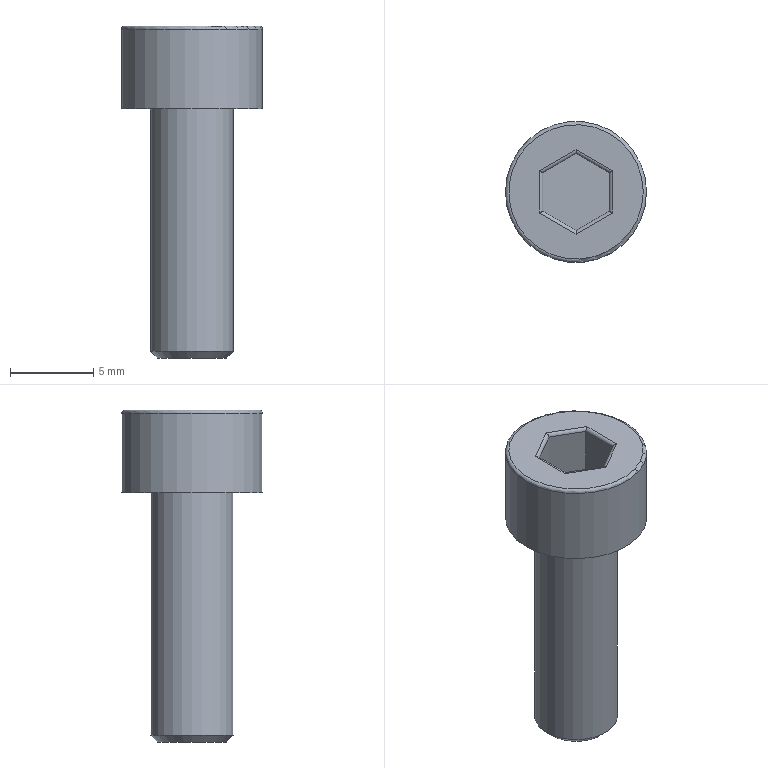Part | STEP file | 200 mesh_id130_x | 1 solid | 20 faces | box 8.5 x 8.5 x 20 mm | volume 535.142 mm3 | plane 10 | cylinder 8 | torus 1 | cone 1 | commonest cylinder face diameters 0.4 x6 5 x1 8.5 x1
STEP:
#1=CARTESIAN_POINT('',(-17018.123,-3964.269,66.658));
#2=VERTEX_POINT('',#1);
#3=CARTESIAN_POINT('',(-17015.623,-3964.269,66.658));
#4=DIRECTION('',(0.,0.,1.));
#5=DIRECTION('',(-1.,0.,0.));
#6=AXIS2_PLACEMENT_3D('',#3,#4,#5);
#7=CIRCLE('',#6,2.5);
#8=EDGE_CURVE('',#2,#2,#7,.T.);
#9=ORIENTED_EDGE('',*,*,#8,.T.);
#10=EDGE_LOOP('',(#9));
#11=FACE_BOUND('',#10,.T.);
#12=CARTESIAN_POINT('',(-17018.123,-3964.269,81.258));
#13=VERTEX_POINT('',#12);
#14=CARTESIAN_POINT('',(-17015.623,-3964.269,81.258));
#15=DIRECTION('',(0.,0.,1.));
#16=DIRECTION('',(-1.,0.,0.));
#17=AXIS2_PLACEMENT_3D('',#14,#15,#16);
#18=CIRCLE('',#17,2.5);
#19=EDGE_CURVE('',#13,#13,#18,.T.);
#20=ORIENTED_EDGE('',*,*,#19,.F.);
#21=EDGE_LOOP('',(#20));
#22=FACE_BOUND('',#21,.T.);
#23=CARTESIAN_POINT('',(-17015.623,-3964.269,81.258));
#24=DIRECTION('',(0.,0.,-1.));
#25=DIRECTION('',(1.,0.,0.));
#26=AXIS2_PLACEMENT_3D('',#23,#24,#25);
#27=CYLINDRICAL_SURFACE('',#26,2.5);
#28=ADVANCED_FACE('',(#11,#22),#27,.T.);
#29=CARTESIAN_POINT('',(-17015.623,-3961.729,86.258));
#30=VERTEX_POINT('',#29);
#31=CARTESIAN_POINT('',(-17013.423,-3962.999,86.258));
#32=VERTEX_POINT('',#31);
#33=CARTESIAN_POINT('',(-17013.523,-3962.941,86.258));
#34=DIRECTION('',(0.866,-0.5,0.));
#35=VECTOR('',#34,1.);
#36=LINE('',#33,#35);
#37=EDGE_CURVE('',#30,#32,#36,.T.);
#38=ORIENTED_EDGE('',*,*,#37,.T.);
#39=CARTESIAN_POINT('',(-17013.423,-3965.539,86.258));
#40=VERTEX_POINT('',#39);
#41=CARTESIAN_POINT('',(-17013.423,-3965.424,86.258));
#42=DIRECTION('',(0.,-1.,0.));
#43=VECTOR('',#42,1.);
#44=LINE('',#41,#43);
#45=EDGE_CURVE('',#32,#40,#44,.T.);
#46=ORIENTED_EDGE('',*,*,#45,.T.);
#47=CARTESIAN_POINT('',(-17015.623,-3966.81,86.258));
#48=VERTEX_POINT('',#47);
#49=CARTESIAN_POINT('',(-17015.523,-3966.752,86.258));
#50=DIRECTION('',(-0.866,-0.5,0.));
#51=VECTOR('',#50,1.);
#52=LINE('',#49,#51);
#53=EDGE_CURVE('',#40,#48,#52,.T.);
#54=ORIENTED_EDGE('',*,*,#53,.T.);
#55=CARTESIAN_POINT('',(-17017.823,-3965.539,86.258));
#56=VERTEX_POINT('',#55);
#57=CARTESIAN_POINT('',(-17017.723,-3965.597,86.258));
#58=DIRECTION('',(-0.866,0.5,0.));
#59=VECTOR('',#58,1.);
#60=LINE('',#57,#59);
#61=EDGE_CURVE('',#48,#56,#60,.T.);
#62=ORIENTED_EDGE('',*,*,#61,.T.);
#63=CARTESIAN_POINT('',(-17017.823,-3962.999,86.258));
#64=VERTEX_POINT('',#63);
#65=CARTESIAN_POINT('',(-17017.823,-3963.114,86.258));
#66=DIRECTION('',(0.,1.,0.));
#67=VECTOR('',#66,1.);
#68=LINE('',#65,#67);
#69=EDGE_CURVE('',#56,#64,#68,.T.);
#70=ORIENTED_EDGE('',*,*,#69,.T.);
#71=CARTESIAN_POINT('',(-17015.723,-3961.787,86.258));
#72=DIRECTION('',(0.866,0.5,0.));
#73=VECTOR('',#72,1.);
#74=LINE('',#71,#73);
#75=EDGE_CURVE('',#64,#30,#74,.T.);
#76=ORIENTED_EDGE('',*,*,#75,.T.);
#77=EDGE_LOOP('',(#38,#46,#54,#62,#70,#76));
#78=FACE_BOUND('',#77,.T.);
#79=CARTESIAN_POINT('',(-17011.573,-3964.269,86.258));
#80=VERTEX_POINT('',#79);
#81=CARTESIAN_POINT('',(-17015.623,-3964.269,86.258));
#82=DIRECTION('',(0.,0.,1.));
#83=DIRECTION('',(1.,0.,0.));
#84=AXIS2_PLACEMENT_3D('',#81,#82,#83);
#85=CIRCLE('',#84,4.05);
#86=EDGE_CURVE('',#80,#80,#85,.T.);
#87=ORIENTED_EDGE('',*,*,#86,.T.);
#88=EDGE_LOOP('',(#87));
#89=FACE_BOUND('',#88,.T.);
#90=CARTESIAN_POINT('',(-17015.623,-3964.269,86.258));
#91=DIRECTION('',(0.,0.,1.));
#92=DIRECTION('',(1.,0.,0.));
#93=AXIS2_PLACEMENT_3D('',#90,#91,#92);
#94=PLANE('',#93);
#95=ADVANCED_FACE('',(#78,#89),#94,.T.);
#96=ORIENTED_EDGE('',*,*,#19,.T.);
#97=EDGE_LOOP('',(#96));
#98=FACE_BOUND('',#97,.T.);
#99=CARTESIAN_POINT('',(-17011.373,-3964.269,81.258));
#100=VERTEX_POINT('',#99);
#101=CARTESIAN_POINT('',(-17015.623,-3964.269,81.258));
#102=DIRECTION('',(0.,0.,1.));
#103=DIRECTION('',(1.,0.,0.));
#104=AXIS2_PLACEMENT_3D('',#101,#102,#103);
#105=CIRCLE('',#104,4.25);
#106=EDGE_CURVE('',#100,#100,#105,.T.);
#107=ORIENTED_EDGE('',*,*,#106,.F.);
#108=EDGE_LOOP('',(#107));
#109=FACE_BOUND('',#108,.T.);
#110=CARTESIAN_POINT('',(-17015.623,-3964.269,81.258));
#111=DIRECTION('',(0.,0.,-1.));
#112=DIRECTION('',(-1.,0.,0.));
#113=AXIS2_PLACEMENT_3D('',#110,#111,#112);
#114=PLANE('',#113);
#115=ADVANCED_FACE('',(#98,#109),#114,.T.);
#116=CARTESIAN_POINT('',(-17011.373,-3964.269,86.058));
#117=VERTEX_POINT('',#116);
#118=CARTESIAN_POINT('',(-17015.623,-3964.269,86.058));
#119=DIRECTION('',(0.,0.,-1.));
#120=DIRECTION('',(1.,0.,0.));
#121=AXIS2_PLACEMENT_3D('',#118,#119,#120);
#122=CIRCLE('',#121,4.25);
#123=EDGE_CURVE('',#117,#117,#122,.T.);
#124=ORIENTED_EDGE('',*,*,#123,.T.);
#125=EDGE_LOOP('',(#124));
#126=FACE_BOUND('',#125,.T.);
#127=ORIENTED_EDGE('',*,*,#106,.T.);
#128=EDGE_LOOP('',(#127));
#129=FACE_BOUND('',#128,.T.);
#130=CARTESIAN_POINT('',(-17015.623,-3964.269,81.258));
#131=DIRECTION('',(0.,0.,1.));
#132=DIRECTION('',(1.,0.,0.));
#133=AXIS2_PLACEMENT_3D('',#130,#131,#132);
#134=CYLINDRICAL_SURFACE('',#133,4.25);
#135=ADVANCED_FACE('',(#126,#129),#134,.T.);
#136=CARTESIAN_POINT('',(-17013.623,-3963.114,86.058));
#137=VERTEX_POINT('',#136);
#138=CARTESIAN_POINT('',(-17013.623,-3963.114,83.258));
#139=VERTEX_POINT('',#138);
#140=CARTESIAN_POINT('',(-17013.623,-3963.114,83.258));
#141=DIRECTION('',(0.,0.,-1.));
#142=VECTOR('',#141,1.);
#143=LINE('',#140,#142);
#144=EDGE_CURVE('',#137,#139,#143,.T.);
#145=ORIENTED_EDGE('',*,*,#144,.F.);
#146=CARTESIAN_POINT('',(-17015.623,-3961.96,86.058));
#147=VERTEX_POINT('',#146);
#148=CARTESIAN_POINT('',(-17015.623,-3961.96,86.058));
#149=DIRECTION('',(-0.866,0.5,0.));
#150=VECTOR('',#149,1.);
#151=LINE('',#148,#150);
#152=EDGE_CURVE('',#137,#147,#151,.T.);
#153=ORIENTED_EDGE('',*,*,#152,.T.);
#154=CARTESIAN_POINT('',(-17015.623,-3961.96,83.258));
#155=VERTEX_POINT('',#154);
#156=CARTESIAN_POINT('',(-17015.623,-3961.96,83.258));
#157=DIRECTION('',(0.,0.,-1.));
#158=VECTOR('',#157,1.);
#159=LINE('',#156,#158);
#160=EDGE_CURVE('',#147,#155,#159,.T.);
#161=ORIENTED_EDGE('',*,*,#160,.T.);
#162=CARTESIAN_POINT('',(-17013.623,-3963.114,83.258));
#163=DIRECTION('',(0.866,-0.5,0.));
#164=VECTOR('',#163,1.);
#165=LINE('',#162,#164);
#166=EDGE_CURVE('',#155,#139,#165,.T.);
#167=ORIENTED_EDGE('',*,*,#166,.T.);
#168=EDGE_LOOP('',(#145,#153,#161,#167));
#169=FACE_OUTER_BOUND('',#168,.T.);
#170=CARTESIAN_POINT('',(-17013.623,-3963.114,83.258));
#171=DIRECTION('',(0.5,0.866,0.));
#172=DIRECTION('',(-0.866,0.5,0.));
#173=AXIS2_PLACEMENT_3D('',#170,#171,#172);
#174=PLANE('',#173);
#175=ADVANCED_FACE('',(#169),#174,.F.);
#176=ORIENTED_EDGE('',*,*,#160,.F.);
#177=CARTESIAN_POINT('',(-17017.623,-3963.114,86.058));
#178=VERTEX_POINT('',#177);
#179=CARTESIAN_POINT('',(-17017.623,-3963.114,86.058));
#180=DIRECTION('',(-0.866,-0.5,0.));
#181=VECTOR('',#180,1.);
#182=LINE('',#179,#181);
#183=EDGE_CURVE('',#147,#178,#182,.T.);
#184=ORIENTED_EDGE('',*,*,#183,.T.);
#185=CARTESIAN_POINT('',(-17017.623,-3963.114,83.258));
#186=VERTEX_POINT('',#185);
#187=CARTESIAN_POINT('',(-17017.623,-3963.114,83.258));
#188=DIRECTION('',(0.,0.,-1.));
#189=VECTOR('',#188,1.);
#190=LINE('',#187,#189);
#191=EDGE_CURVE('',#178,#186,#190,.T.);
#192=ORIENTED_EDGE('',*,*,#191,.T.);
#193=CARTESIAN_POINT('',(-17015.623,-3961.96,83.258));
#194=DIRECTION('',(0.866,0.5,0.));
#195=VECTOR('',#194,1.);
#196=LINE('',#193,#195);
#197=EDGE_CURVE('',#186,#155,#196,.T.);
#198=ORIENTED_EDGE('',*,*,#197,.T.);
#199=EDGE_LOOP('',(#176,#184,#192,#198));
#200=FACE_OUTER_BOUND('',#199,.T.);
#201=CARTESIAN_POINT('',(-17015.623,-3961.96,83.258));
#202=DIRECTION('',(-0.5,0.866,0.));
#203=DIRECTION('',(-0.866,-0.5,0.));
#204=AXIS2_PLACEMENT_3D('',#201,#202,#203);
#205=PLANE('',#204);
#206=ADVANCED_FACE('',(#200),#205,.F.);
#207=ORIENTED_EDGE('',*,*,#191,.F.);
#208=CARTESIAN_POINT('',(-17017.623,-3965.424,86.058));
#209=VERTEX_POINT('',#208);
#210=CARTESIAN_POINT('',(-17017.623,-3965.424,86.058));
#211=DIRECTION('',(0.,-1.,0.));
#212=VECTOR('',#211,1.);
#213=LINE('',#210,#212);
#214=EDGE_CURVE('',#178,#209,#213,.T.);
#215=ORIENTED_EDGE('',*,*,#214,.T.);
#216=CARTESIAN_POINT('',(-17017.623,-3965.424,83.258));
#217=VERTEX_POINT('',#216);
#218=CARTESIAN_POINT('',(-17017.623,-3965.424,83.258));
#219=DIRECTION('',(0.,0.,-1.));
#220=VECTOR('',#219,1.);
#221=LINE('',#218,#220);
#222=EDGE_CURVE('',#209,#217,#221,.T.);
#223=ORIENTED_EDGE('',*,*,#222,.T.);
#224=CARTESIAN_POINT('',(-17017.623,-3963.114,83.258));
#225=DIRECTION('',(0.,1.,0.));
#226=VECTOR('',#225,1.);
#227=LINE('',#224,#226);
#228=EDGE_CURVE('',#217,#186,#227,.T.);
#229=ORIENTED_EDGE('',*,*,#228,.T.);
#230=EDGE_LOOP('',(#207,#215,#223,#229));
#231=FACE_OUTER_BOUND('',#230,.T.);
#232=CARTESIAN_POINT('',(-17017.623,-3963.114,83.258));
#233=DIRECTION('',(-1.,0.,0.));
#234=DIRECTION('',(0.,0.,1.));
#235=AXIS2_PLACEMENT_3D('',#232,#233,#234);
#236=PLANE('',#235);
#237=ADVANCED_FACE('',(#231),#236,.F.);
#238=ORIENTED_EDGE('',*,*,#222,.F.);
#239=CARTESIAN_POINT('',(-17015.623,-3966.579,86.058));
#240=VERTEX_POINT('',#239);
#241=CARTESIAN_POINT('',(-17015.623,-3966.579,86.058));
#242=DIRECTION('',(0.866,-0.5,0.));
#243=VECTOR('',#242,1.);
#244=LINE('',#241,#243);
#245=EDGE_CURVE('',#209,#240,#244,.T.);
#246=ORIENTED_EDGE('',*,*,#245,.T.);
#247=CARTESIAN_POINT('',(-17015.623,-3966.579,83.258));
#248=VERTEX_POINT('',#247);
#249=CARTESIAN_POINT('',(-17015.623,-3966.579,83.258));
#250=DIRECTION('',(0.,0.,-1.));
#251=VECTOR('',#250,1.);
#252=LINE('',#249,#251);
#253=EDGE_CURVE('',#240,#248,#252,.T.);
#254=ORIENTED_EDGE('',*,*,#253,.T.);
#255=CARTESIAN_POINT('',(-17017.623,-3965.424,83.258));
#256=DIRECTION('',(-0.866,0.5,0.));
#257=VECTOR('',#256,1.);
#258=LINE('',#255,#257);
#259=EDGE_CURVE('',#248,#217,#258,.T.);
#260=ORIENTED_EDGE('',*,*,#259,.T.);
#261=EDGE_LOOP('',(#238,#246,#254,#260));
#262=FACE_OUTER_BOUND('',#261,.T.);
#263=CARTESIAN_POINT('',(-17017.623,-3965.424,83.258));
#264=DIRECTION('',(-0.5,-0.866,0.));
#265=DIRECTION('',(0.866,-0.5,0.));
#266=AXIS2_PLACEMENT_3D('',#263,#264,#265);
#267=PLANE('',#266);
#268=ADVANCED_FACE('',(#262),#267,.F.);
#269=ORIENTED_EDGE('',*,*,#253,.F.);
#270=CARTESIAN_POINT('',(-17013.623,-3965.424,86.058));
#271=VERTEX_POINT('',#270);
#272=CARTESIAN_POINT('',(-17013.623,-3965.424,86.058));
#273=DIRECTION('',(0.866,0.5,0.));
#274=VECTOR('',#273,1.);
#275=LINE('',#272,#274);
#276=EDGE_CURVE('',#240,#271,#275,.T.);
#277=ORIENTED_EDGE('',*,*,#276,.T.);
#278=CARTESIAN_POINT('',(-17013.623,-3965.424,83.258));
#279=VERTEX_POINT('',#278);
#280=CARTESIAN_POINT('',(-17013.623,-3965.424,83.258));
#281=DIRECTION('',(0.,0.,-1.));
#282=VECTOR('',#281,1.);
#283=LINE('',#280,#282);
#284=EDGE_CURVE('',#271,#279,#283,.T.);
#285=ORIENTED_EDGE('',*,*,#284,.T.);
#286=CARTESIAN_POINT('',(-17015.623,-3966.579,83.258));
#287=DIRECTION('',(-0.866,-0.5,0.));
#288=VECTOR('',#287,1.);
#289=LINE('',#286,#288);
#290=EDGE_CURVE('',#279,#248,#289,.T.);
#291=ORIENTED_EDGE('',*,*,#290,.T.);
#292=EDGE_LOOP('',(#269,#277,#285,#291));
#293=FACE_OUTER_BOUND('',#292,.T.);
#294=CARTESIAN_POINT('',(-17015.623,-3966.579,83.258));
#295=DIRECTION('',(0.5,-0.866,0.));
#296=DIRECTION('',(0.866,0.5,0.));
#297=AXIS2_PLACEMENT_3D('',#294,#295,#296);
#298=PLANE('',#297);
#299=ADVANCED_FACE('',(#293),#298,.F.);
#300=ORIENTED_EDGE('',*,*,#284,.F.);
#301=CARTESIAN_POINT('',(-17013.623,-3963.114,86.058));
#302=DIRECTION('',(0.,1.,0.));
#303=VECTOR('',#302,1.);
#304=LINE('',#301,#303);
#305=EDGE_CURVE('',#271,#137,#304,.T.);
#306=ORIENTED_EDGE('',*,*,#305,.T.);
#307=ORIENTED_EDGE('',*,*,#144,.T.);
#308=CARTESIAN_POINT('',(-17013.623,-3965.424,83.258));
#309=DIRECTION('',(0.,-1.,0.));
#310=VECTOR('',#309,1.);
#311=LINE('',#308,#310);
#312=EDGE_CURVE('',#139,#279,#311,.T.);
#313=ORIENTED_EDGE('',*,*,#312,.T.);
#314=EDGE_LOOP('',(#300,#306,#307,#313));
#315=FACE_OUTER_BOUND('',#314,.T.);
#316=CARTESIAN_POINT('',(-17013.623,-3965.424,83.258));
#317=DIRECTION('',(1.,0.,0.));
#318=DIRECTION('',(0.,0.,-1.));
#319=AXIS2_PLACEMENT_3D('',#316,#317,#318);
#320=PLANE('',#319);
#321=ADVANCED_FACE('',(#315),#320,.F.);
#322=ORIENTED_EDGE('',*,*,#166,.F.);
#323=ORIENTED_EDGE('',*,*,#197,.F.);
#324=ORIENTED_EDGE('',*,*,#228,.F.);
#325=ORIENTED_EDGE('',*,*,#259,.F.);
#326=ORIENTED_EDGE('',*,*,#290,.F.);
#327=ORIENTED_EDGE('',*,*,#312,.F.);
#328=EDGE_LOOP('',(#322,#323,#324,#325,#326,#327));
#329=FACE_OUTER_BOUND('',#328,.T.);
#330=CARTESIAN_POINT('',(-95.,0.,83.258));
#331=DIRECTION('',(0.,0.,1.));
#332=DIRECTION('',(1.,0.,0.));
#333=AXIS2_PLACEMENT_3D('',#330,#331,#332);
#334=PLANE('',#333);
#335=ADVANCED_FACE('',(#329),#334,.T.);
#336=ORIENTED_EDGE('',*,*,#86,.F.);
#337=EDGE_LOOP('',(#336));
#338=FACE_BOUND('',#337,.T.);
#339=ORIENTED_EDGE('',*,*,#123,.F.);
#340=EDGE_LOOP('',(#339));
#341=FACE_BOUND('',#340,.T.);
#342=CARTESIAN_POINT('',(-17015.623,-3964.269,86.058));
#343=DIRECTION('',(0.,0.,1.));
#344=DIRECTION('',(1.,0.,0.));
#345=AXIS2_PLACEMENT_3D('',#342,#343,#344);
#346=TOROIDAL_SURFACE('',#345,4.05,0.2);
#347=ADVANCED_FACE('',(#338,#341),#346,.T.);
#348=CARTESIAN_POINT('',(-17017.823,-3962.999,86.058));
#349=DIRECTION('',(0.5,0.866,0.));
#350=DIRECTION('',(-0.866,0.5,0.));
#351=AXIS2_PLACEMENT_3D('',#348,#349,#350);
#352=ELLIPSE('',#351,0.2309,0.2);
#353=EDGE_CURVE('',#64,#178,#352,.T.);
#354=ORIENTED_EDGE('',*,*,#353,.F.);
#355=ORIENTED_EDGE('',*,*,#69,.F.);
#356=CARTESIAN_POINT('',(-17017.823,-3965.539,86.058));
#357=DIRECTION('',(0.5,-0.866,0.));
#358=DIRECTION('',(-0.866,-0.5,0.));
#359=AXIS2_PLACEMENT_3D('',#356,#357,#358);
#360=ELLIPSE('',#359,0.2309,0.2);
#361=EDGE_CURVE('',#209,#56,#360,.T.);
#362=ORIENTED_EDGE('',*,*,#361,.F.);
#363=ORIENTED_EDGE('',*,*,#214,.F.);
#364=EDGE_LOOP('',(#354,#355,#362,#363));
#365=FACE_OUTER_BOUND('',#364,.T.);
#366=CARTESIAN_POINT('',(-17017.823,-3963.114,86.058));
#367=DIRECTION('',(0.,1.,0.));
#368=DIRECTION('',(0.,0.,1.));
#369=AXIS2_PLACEMENT_3D('',#366,#367,#368);
#370=CYLINDRICAL_SURFACE('',#369,0.2);
#371=ADVANCED_FACE('',(#365),#370,.T.);
#372=ORIENTED_EDGE('',*,*,#361,.T.);
#373=ORIENTED_EDGE('',*,*,#61,.F.);
#374=CARTESIAN_POINT('',(-17015.623,-3966.81,86.058));
#375=DIRECTION('',(1.,0.,0.));
#376=DIRECTION('',(0.,-1.,0.));
#377=AXIS2_PLACEMENT_3D('',#374,#375,#376);
#378=ELLIPSE('',#377,0.2309,0.2);
#379=EDGE_CURVE('',#240,#48,#378,.T.);
#380=ORIENTED_EDGE('',*,*,#379,.F.);
#381=ORIENTED_EDGE('',*,*,#245,.F.);
#382=EDGE_LOOP('',(#372,#373,#380,#381));
#383=FACE_OUTER_BOUND('',#382,.T.);
#384=CARTESIAN_POINT('',(-17017.723,-3965.597,86.058));
#385=DIRECTION('',(-0.866,0.5,0.));
#386=DIRECTION('',(-0.5,-0.866,0.));
#387=AXIS2_PLACEMENT_3D('',#384,#385,#386);
#388=CYLINDRICAL_SURFACE('',#387,0.2);
#389=ADVANCED_FACE('',(#383),#388,.T.);
#390=ORIENTED_EDGE('',*,*,#353,.T.);
#391=ORIENTED_EDGE('',*,*,#183,.F.);
#392=CARTESIAN_POINT('',(-17015.623,-3961.729,86.058));
#393=DIRECTION('',(1.,0.,0.));
#394=DIRECTION('',(0.,1.,0.));
#395=AXIS2_PLACEMENT_3D('',#392,#393,#394);
#396=ELLIPSE('',#395,0.2309,0.2);
#397=EDGE_CURVE('',#30,#147,#396,.T.);
#398=ORIENTED_EDGE('',*,*,#397,.F.);
#399=ORIENTED_EDGE('',*,*,#75,.F.);
#400=EDGE_LOOP('',(#390,#391,#398,#399));
#401=FACE_OUTER_BOUND('',#400,.T.);
#402=CARTESIAN_POINT('',(-17015.723,-3961.787,86.058));
#403=DIRECTION('',(0.866,0.5,0.));
#404=DIRECTION('',(-0.5,0.866,0.));
#405=AXIS2_PLACEMENT_3D('',#402,#403,#404);
#406=CYLINDRICAL_SURFACE('',#405,0.2);
#407=ADVANCED_FACE('',(#401),#406,.T.);
#408=ORIENTED_EDGE('',*,*,#379,.T.);
#409=ORIENTED_EDGE('',*,*,#53,.F.);
#410=CARTESIAN_POINT('',(-17013.423,-3965.539,86.058));
#411=DIRECTION('',(0.5,0.866,0.));
#412=DIRECTION('',(0.866,-0.5,0.));
#413=AXIS2_PLACEMENT_3D('',#410,#411,#412);
#414=ELLIPSE('',#413,0.2309,0.2);
#415=EDGE_CURVE('',#271,#40,#414,.T.);
#416=ORIENTED_EDGE('',*,*,#415,.F.);
#417=ORIENTED_EDGE('',*,*,#276,.F.);
#418=EDGE_LOOP('',(#408,#409,#416,#417));
#419=FACE_OUTER_BOUND('',#418,.T.);
#420=CARTESIAN_POINT('',(-17015.523,-3966.752,86.058));
#421=DIRECTION('',(-0.866,-0.5,0.));
#422=DIRECTION('',(0.5,-0.866,0.));
#423=AXIS2_PLACEMENT_3D('',#420,#421,#422);
#424=CYLINDRICAL_SURFACE('',#423,0.2);
#425=ADVANCED_FACE('',(#419),#424,.T.);
#426=ORIENTED_EDGE('',*,*,#397,.T.);
#427=ORIENTED_EDGE('',*,*,#152,.F.);
#428=CARTESIAN_POINT('',(-17013.423,-3962.999,86.058));
#429=DIRECTION('',(0.5,-0.866,0.));
#430=DIRECTION('',(-0.866,-0.5,0.));
#431=AXIS2_PLACEMENT_3D('',#428,#429,#430);
#432=ELLIPSE('',#431,0.2309,0.2);
#433=EDGE_CURVE('',#32,#137,#432,.T.);
#434=ORIENTED_EDGE('',*,*,#433,.F.);
#435=ORIENTED_EDGE('',*,*,#37,.F.);
#436=EDGE_LOOP('',(#426,#427,#434,#435));
#437=FACE_OUTER_BOUND('',#436,.T.);
#438=CARTESIAN_POINT('',(-17013.523,-3962.941,86.058));
#439=DIRECTION('',(0.866,-0.5,0.));
#440=DIRECTION('',(0.5,0.866,0.));
#441=AXIS2_PLACEMENT_3D('',#438,#439,#440);
#442=CYLINDRICAL_SURFACE('',#441,0.2);
#443=ADVANCED_FACE('',(#437),#442,.T.);
#444=ORIENTED_EDGE('',*,*,#415,.T.);
#445=ORIENTED_EDGE('',*,*,#45,.F.);
#446=ORIENTED_EDGE('',*,*,#433,.T.);
#447=ORIENTED_EDGE('',*,*,#305,.F.);
#448=EDGE_LOOP('',(#444,#445,#446,#447));
#449=FACE_OUTER_BOUND('',#448,.T.);
#450=CARTESIAN_POINT('',(-17013.423,-3965.424,86.058));
#451=DIRECTION('',(0.,-1.,0.));
#452=DIRECTION('',(0.,0.,-1.));
#453=AXIS2_PLACEMENT_3D('',#450,#451,#452);
#454=CYLINDRICAL_SURFACE('',#453,0.2);
#455=ADVANCED_FACE('',(#449),#454,.T.);
#456=CARTESIAN_POINT('',(-17017.723,-3964.269,66.258));
#457=VERTEX_POINT('',#456);
#458=CARTESIAN_POINT('',(-17015.623,-3964.269,66.258));
#459=DIRECTION('',(0.,0.,-1.));
#460=DIRECTION('',(-1.,0.,0.));
#461=AXIS2_PLACEMENT_3D('',#458,#459,#460);
#462=CIRCLE('',#461,2.1);
#463=EDGE_CURVE('',#457,#457,#462,.T.);
#464=ORIENTED_EDGE('',*,*,#463,.T.);
#465=EDGE_LOOP('',(#464));
#466=FACE_OUTER_BOUND('',#465,.T.);
#467=CARTESIAN_POINT('',(-17015.623,-3964.269,66.258));
#468=DIRECTION('',(0.,0.,-1.));
#469=DIRECTION('',(-1.,0.,0.));
#470=AXIS2_PLACEMENT_3D('',#467,#468,#469);
#471=PLANE('',#470);
#472=ADVANCED_FACE('',(#466),#471,.T.);
#473=ORIENTED_EDGE('',*,*,#463,.F.);
#474=EDGE_LOOP('',(#473));
#475=FACE_BOUND('',#474,.T.);
#476=ORIENTED_EDGE('',*,*,#8,.F.);
#477=EDGE_LOOP('',(#476));
#478=FACE_BOUND('',#477,.T.);
#479=CARTESIAN_POINT('',(-17015.623,-3964.269,66.658));
#480=DIRECTION('',(0.,0.,1.));
#481=DIRECTION('',(1.,0.,0.));
#482=AXIS2_PLACEMENT_3D('',#479,#480,#481);
#483=CONICAL_SURFACE('',#482,2.5,45.);
#484=ADVANCED_FACE('',(#475,#478),#483,.T.);
#485=CLOSED_SHELL('',(#28,#95,#115,#135,#175,#206,#237,#268,#299,#321,#335,#347,#371,#389,#407,#425,#443,#455,#472,#484));
#486=MANIFOLD_SOLID_BREP('',#485);
#487=(LENGTH_UNIT()NAMED_UNIT(*)SI_UNIT(.MILLI.,.METRE.));
#488=UNCERTAINTY_MEASURE_WITH_UNIT(LENGTH_MEASURE(0.00002),#487,'','');
#489=(NAMED_UNIT(*)PLANE_ANGLE_UNIT()SI_UNIT($,.RADIAN.));
#490=PLANE_ANGLE_MEASURE_WITH_UNIT(PLANE_ANGLE_MEASURE(0.01745),#489);
#491=DIMENSIONAL_EXPONENTS(0.,0.,0.,0.,0.,0.,0.);
#492=(CONVERSION_BASED_UNIT('DEGREE',#490)NAMED_UNIT(#491)PLANE_ANGLE_UNIT());
#493=(NAMED_UNIT(*)SI_UNIT($,.STERADIAN.)SOLID_ANGLE_UNIT());
#494=(GEOMETRIC_REPRESENTATION_CONTEXT(3)GLOBAL_UNCERTAINTY_ASSIGNED_CONTEXT((#488))GLOBAL_UNIT_ASSIGNED_CONTEXT((#487,#492,#493))REPRESENTATION_CONTEXT('',''));
#495=ADVANCED_BREP_SHAPE_REPRESENTATION('',(#486),#494);